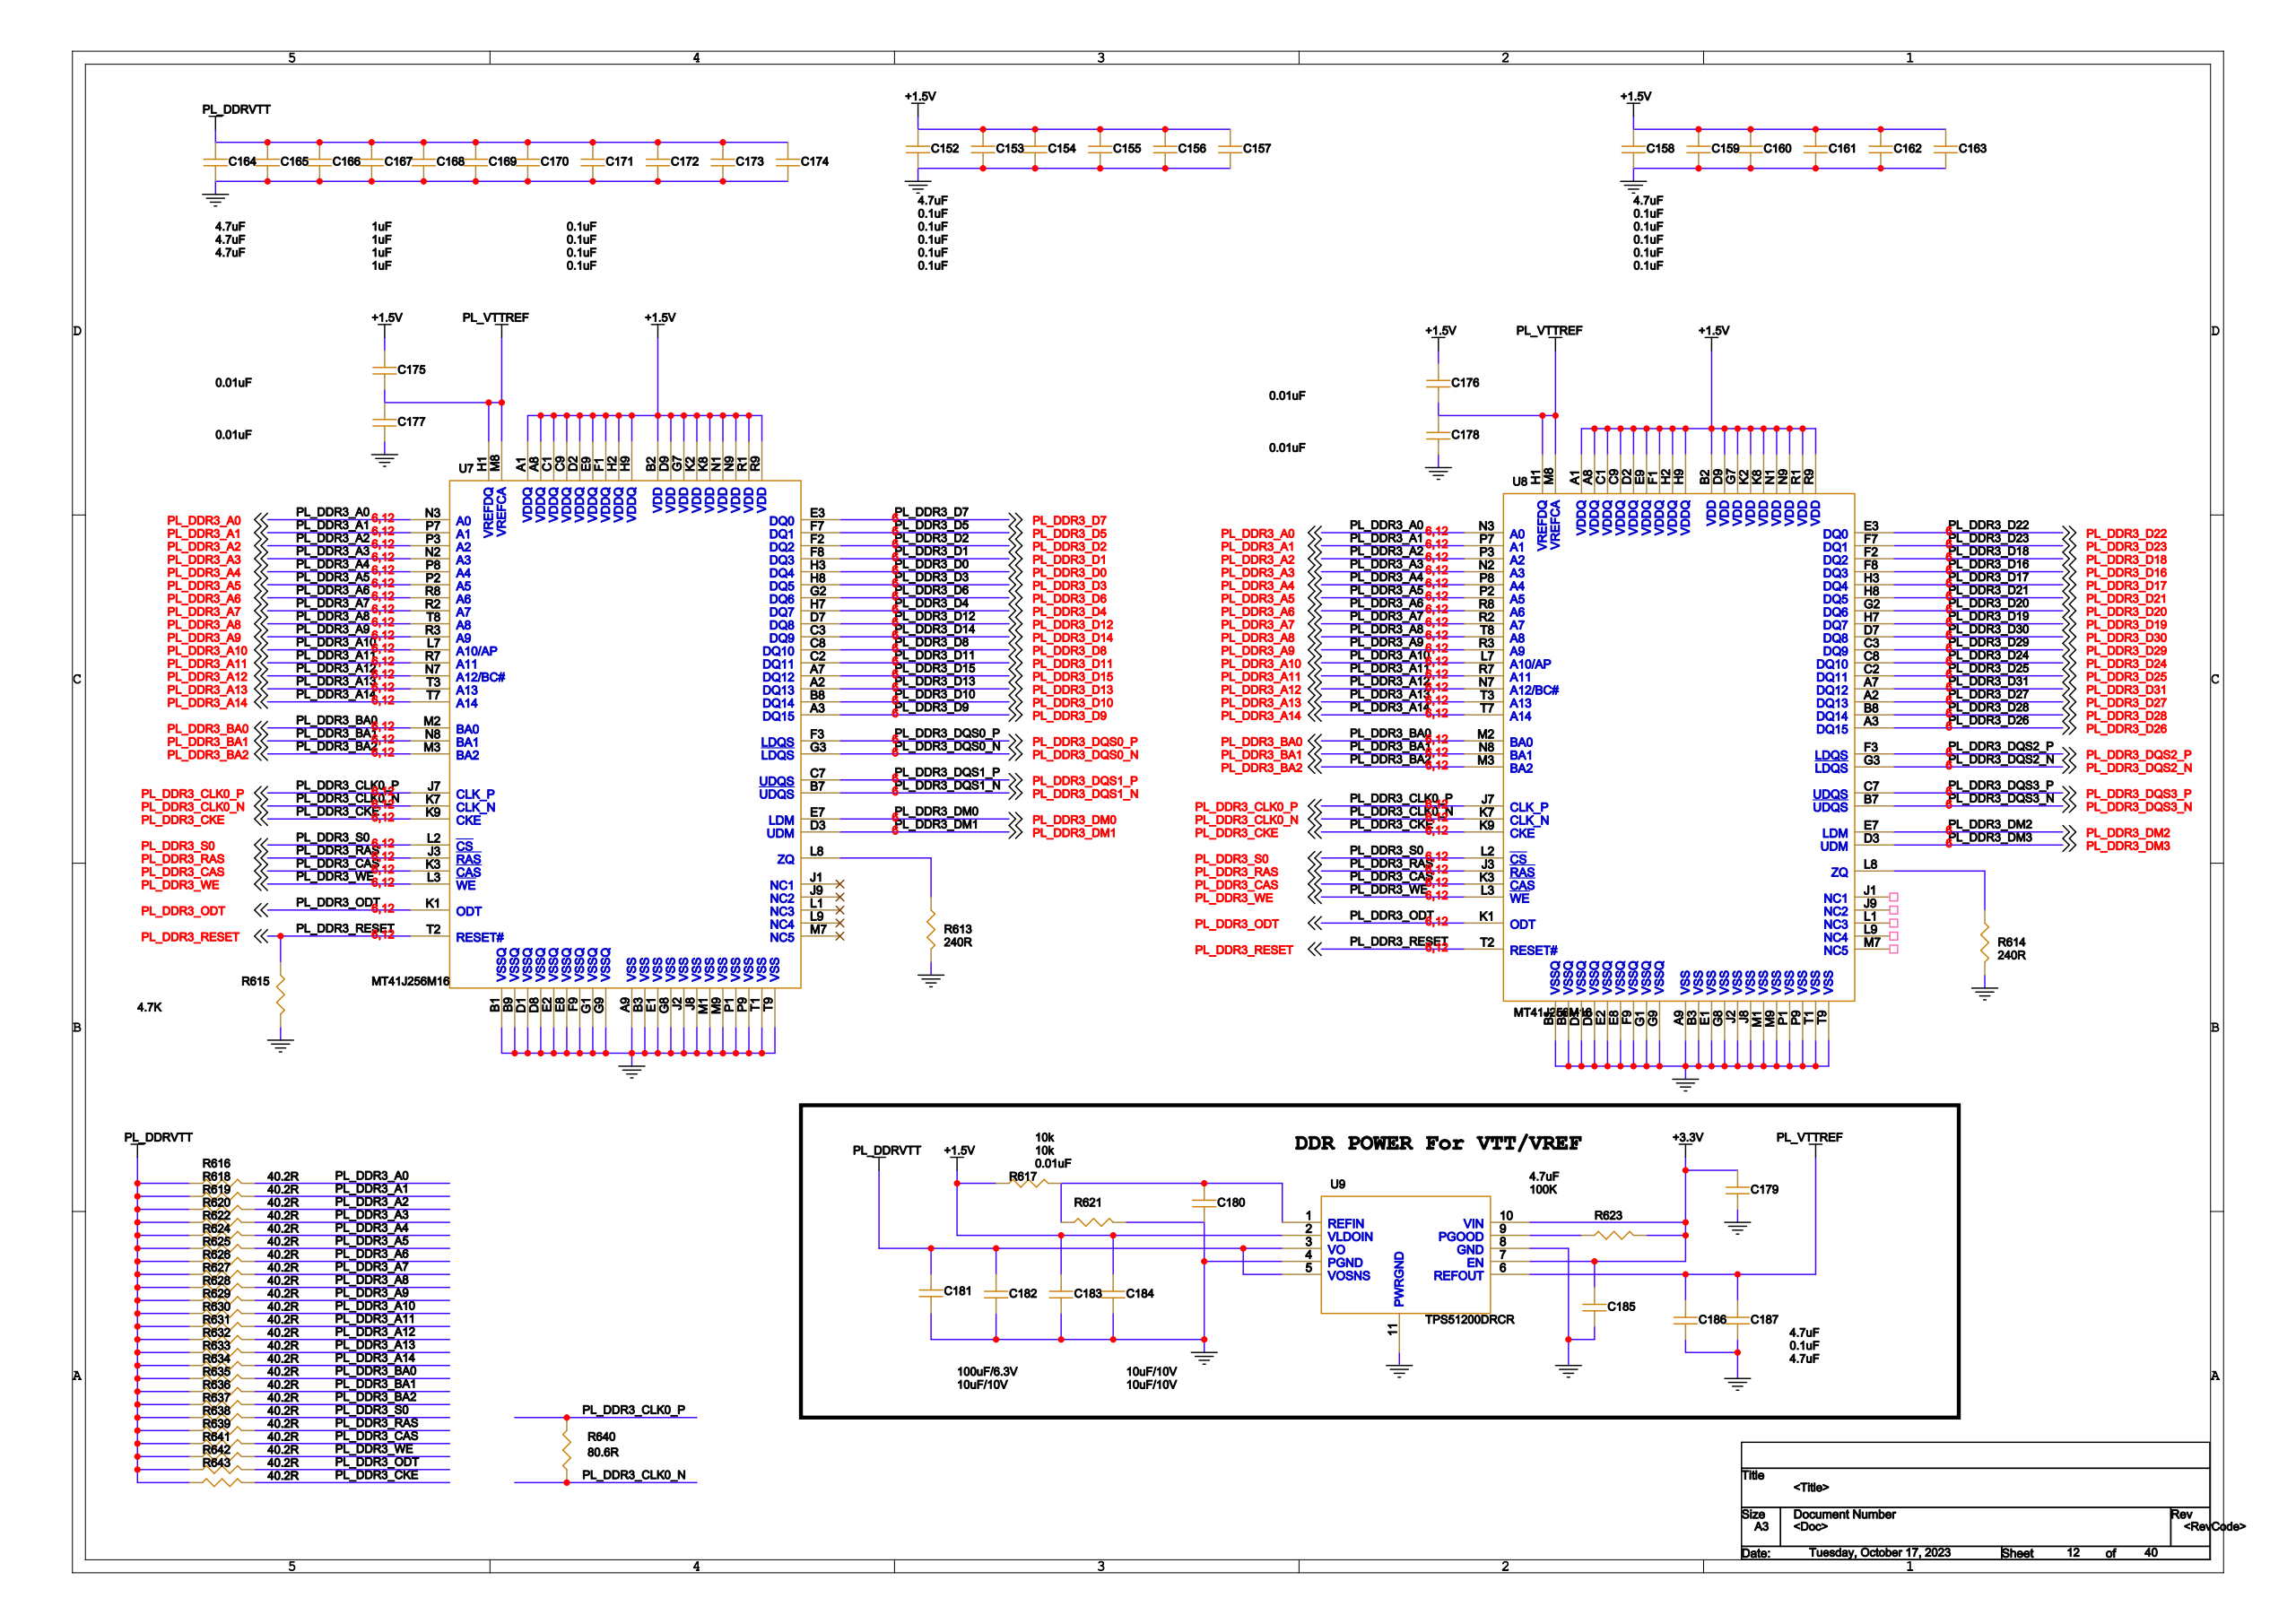Circuit board | Cadence Allegro | 1793 parts | 1223 nets | one sheet of the schematic
Parts on this sheet (reference | value | footprint):
C152 | 4.7uF | C0402
C153 | 0.1uF | C0402
C154 | 0.1uF | C0402
C155 | 0.1uF | C0402
C156 | 0.1uF | C0402
C157 | 0.1uF | C0402
C158 | 4.7uF | C0402
C159 | 0.1uF | C0402
C160 | 0.1uF | C0402
C161 | 0.1uF | C0402
C162 | 0.1uF | C0402
C163 | 0.1uF | C0402
C164 | 4.7uF | C0402
C165 | 4.7uF | C0402
C166 | 4.7uF | C0402
C167 | 1uF | C0402
C168 | 1uF | C0402
C169 | 1uF | C0402
C170 | 1uF | C0402
C171 | 0.1uF | C0402
C172 | 0.1uF | C0402
C173 | 0.1uF | C0402
C174 | 0.1uF | C0402
C175 | 0.01uF | C0402
C176 | 0.01uF | C0402
C177 | 0.01uF | C0402
C178 | 0.01uF | C0402
C179 | 4.7uF | C0402
C180 | 0.01uF | C0402
C181 | 100uF/6.3V | 1206
C182 | 10uF/10V | C0402
C183 | 10uF/10V | C0402
C184 | 10uF/10V | C0402
C185 | 4.7uF | C0402
C186 | 0.1uF | C0402
C187 | 4.7uF | C0402
R613 | 240R | R0402
R614 | 240R | R0402
R615 | 4.7K | R0402
R616 | 40.2R | R0402
R617 | 10k | R0402
R618 | 40.2R | R0402
R619 | 40.2R | R0402
R620 | 40.2R | R0402
R621 | 10k | R0402
R622 | 40.2R | R0402
R623 | 100K | R0402
R624 | 40.2R | R0402
R625 | 40.2R | R0402
R626 | 40.2R | R0402
R627 | 40.2R | R0402
R628 | 40.2R | R0402
R629 | 40.2R | R0402
R630 | 40.2R | R0402
R631 | 40.2R | R0402
R632 | 40.2R | R0402
R633 | 40.2R | R0402
R634 | 40.2R | R0402
R635 | 40.2R | R0402
R636 | 40.2R | R0402
R637 | 40.2R | R0402
R638 | 40.2R | R0402
R639 | 40.2R | R0402
R640 | 80.6R | R0402
R641 | 40.2R | R0402
R642 | 40.2R | R0402
R643 | 40.2R | R0402
U7 | MT41J256M16 | FBGA-96
U8 | MT41J256M16 | FBGA-96
U9 | TPS51200DRCR | TPS51200DRCR
Nets of these parts (net: part-pin ...):
GND: C152-1 C153-1 C154-1 C155-1 C156-1 C157-1 C158-1 C159-1 C160-1 C161-1 C162-1 C163-1 C164-1 C165-1 C166-1 C167-1 C168-1 C169-1 C170-1 C171-1 C172-1 C173-1 C174-1 C177-1 C178-1 C179-1 C180-1 C181-2 C182-1 C183-1 C184-1 C185-1 C186-1 C187-1 R613-1 R614-1 R615-1 R621-1 U9-4 U9-8 U9-11 U7-A9 U7-B1 U7-B3 U7-B9 U7-D1 U7-D8 U7-E1 U7-E2 U7-E8 U7-F9 U7-G1 U7-G8 U7-G9 U7-J2 U7-J8 U7-M1 U7-M9 U7-P1 U7-P9 U7-T1 U7-T9 U8-A9 U8-B1 U8-B3 U8-B9 U8-D1 U8-D8 U8-E1 U8-E2 U8-E8 U8-F9 U8-G1 U8-G8 U8-G9 U8-J2 U8-J8 U8-M1 U8-M9 U8-P1 U8-P9 U8-T1 U8-T9
+1.5V: C152-2 C153-2 C154-2 C155-2 C156-2 C157-2 C158-2 C159-2 C160-2 C161-2 C162-2 C163-2 C175-2 C176-2 C183-2 C184-2 R617-2 U9-2 U7-A1 U7-A8 U7-B2 U7-C1 U7-C9 U7-D2 U7-D9 U7-E9 U7-F1 U7-G7 U7-H2 U7-H9 U7-K2 U7-K8 U7-N1 U7-N9 U7-R1 U7-R9 U8-A1 U8-A8 U8-B2 U8-C1 U8-C9 U8-D2 U8-D9 U8-E9 U8-F1 U8-G7 U8-H2 U8-H9 U8-K2 U8-K8 U8-N1 U8-N9 U8-R1 U8-R9
+3.3V: C179-2 C185-2 R623-1 U9-7 U9-10
PL_DDRVTT: C164-2 C165-2 C166-2 C167-2 C168-2 C169-2 C170-2 C171-2 C172-2 C173-2 C174-2 C181-1 C182-2 R616-2 R618-2 R619-2 R620-2 R622-2 R624-2 R625-2 R626-2 R627-2 R628-2 R629-2 R630-2 R631-2 R632-2 R633-2 R634-2 R635-2 R636-2 R637-2 R638-2 R639-2 R641-2 R642-2 R643-2 U9-3 U9-5
PL_VTTREF: C175-1 C176-1 C177-2 C178-2 C186-2 C187-2 U9-6 U7-H1 U7-M8 U8-H1 U8-M8
PL_DDR3_RESET: R615-2 U7-T2 U8-T2
PL_DDR3_A0: R616-1 U7-N3 U8-N3
PL_DDR3_A1: R618-1 U7-P7 U8-P7
PL_DDR3_A2: R619-1 U7-P3 U8-P3
PL_DDR3_A3: R620-1 U7-N2 U8-N2
PL_DDR3_A4: R622-1 U7-P8 U8-P8
PL_DDR3_A5: R624-1 U7-P2 U8-P2
PL_DDR3_A6: R625-1 U7-R8 U8-R8
PL_DDR3_A7: R626-1 U7-R2 U8-R2
PL_DDR3_A8: R627-1 U7-T8 U8-T8
PL_DDR3_A9: R628-1 U7-R3 U8-R3
PL_DDR3_A10: R629-1 U7-L7 U8-L7
PL_DDR3_A11: R630-1 U7-R7 U8-R7
PL_DDR3_A12: R631-1 U7-N7 U8-N7
PL_DDR3_A13: R632-1 U7-T3 U8-T3
PL_DDR3_A14: R633-1 U7-T7 U8-T7
PL_DDR3_BA0: R634-1 U7-M2 U8-M2
PL_DDR3_BA1: R635-1 U7-N8 U8-N8
PL_DDR3_BA2: R636-1 U7-M3 U8-M3
PL_DDR3_S0: R637-1 U7-L2 U8-L2
PL_DDR3_RAS: R638-1 U7-J3 U8-J3
PL_DDR3_CAS: R639-1 U7-K3 U8-K3
PL_DDR3_WE: R641-1 U7-L3 U8-L3
PL_DDR3_ODT: R642-1 U7-K1 U8-K1
PL_DDR3_CKE: R643-1 U7-K9 U8-K9
PL_DDR3_CLK0_P: R640-1 U7-J7 U8-J7
PL_DDR3_CLK0_N: R640-2 U7-K7 U8-K7
N159276: R613-2 U7-L8
N159326: R614-2 U8-L8
N160090: R623-2 U9-9
N159812: C180-2 R617-1 R621-2 U9-1
PL_DDR3_D9: U7-A3
PL_DDR3_D12: U7-D7
PL_DDR3_D15: U7-A7
PL_DDR3_D8: U7-C8
PL_DDR3_D13: U7-A2
PL_DDR3_DM1: U7-D3
PL_DDR3_D21: U8-H8
PL_DDR3_DM2: U8-E7
PL_DDR3_D19: U8-H7
PL_DDR3_DQS2_N: U8-G3
PL_DDR3_DQS2_P: U8-F3
PL_DDR3_D18: U8-F2
PL_DDR3_D22: U8-E3
PL_DDR3_D23: U8-F7
PL_DDR3_D17: U8-H3
PL_DDR3_D20: U8-G2
PL_DDR3_D16: U8-F8
PL_DDR3_D30: U8-D7
PL_DDR3_D0: U7-H3
PL_DDR3_D2: U7-F2
PL_DDR3_D26: U8-A3
PL_DDR3_D27: U8-A2
PL_DDR3_DQS3_N: U8-B7
PL_DDR3_DQS3_P: U8-C7
PL_DDR3_D28: U8-B8
PL_DDR3_D24: U8-C8
PL_DDR3_DM3: U8-D3
PL_DDR3_D31: U8-A7
PL_DDR3_D25: U8-C2
PL_DDR3_D29: U8-C3
PL_DDR3_D4: U7-H7
PL_DDR3_DM0: U7-E7
PL_DDR3_DQS0_N: U7-G3
PL_DDR3_DQS0_P: U7-F3
PL_DDR3_D1: U7-F8
PL_DDR3_D3: U7-H8
PL_DDR3_D6: U7-G2
PL_DDR3_D7: U7-E3
PL_DDR3_D5: U7-F7
PL_DDR3_D11: U7-C2
PL_DDR3_D14: U7-C3
PL_DDR3_D10: U7-B8
PL_DDR3_DQS1_N: U7-B7
PL_DDR3_DQS1_P: U7-C7